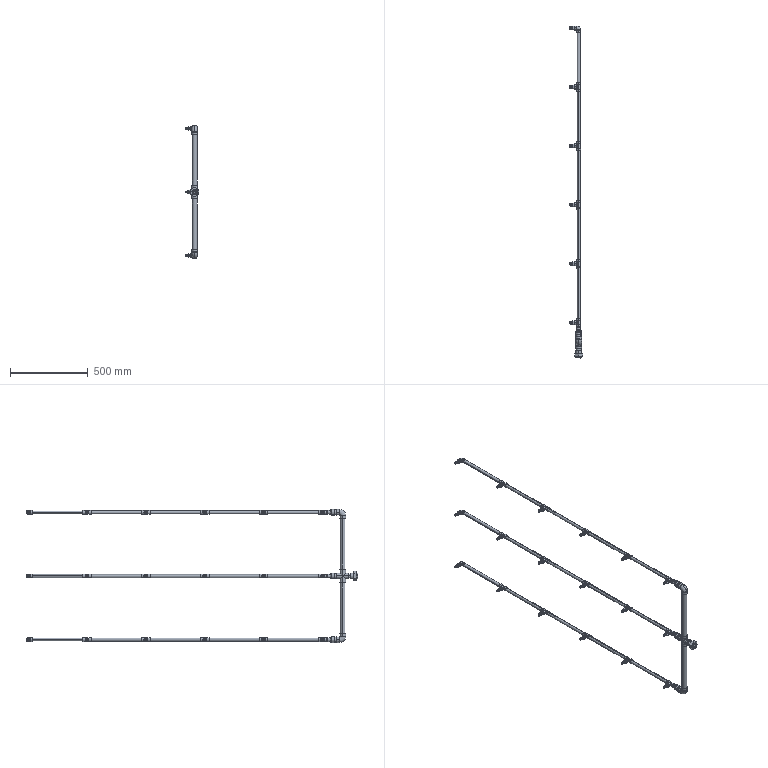Part | SolidWorks | features ReferencePattern 36, LocalLPattern 3 | 85 solids | 1304 faces | box 86.11 x 2140 x 858 mm | volume 1331327 mm3 | plane 688 | cylinder 548 | cone 48 | torus 20 | commonest cylinder face diameters 20 x165 25 x93 10 x72 16 x72 12.384 x36 14 x36